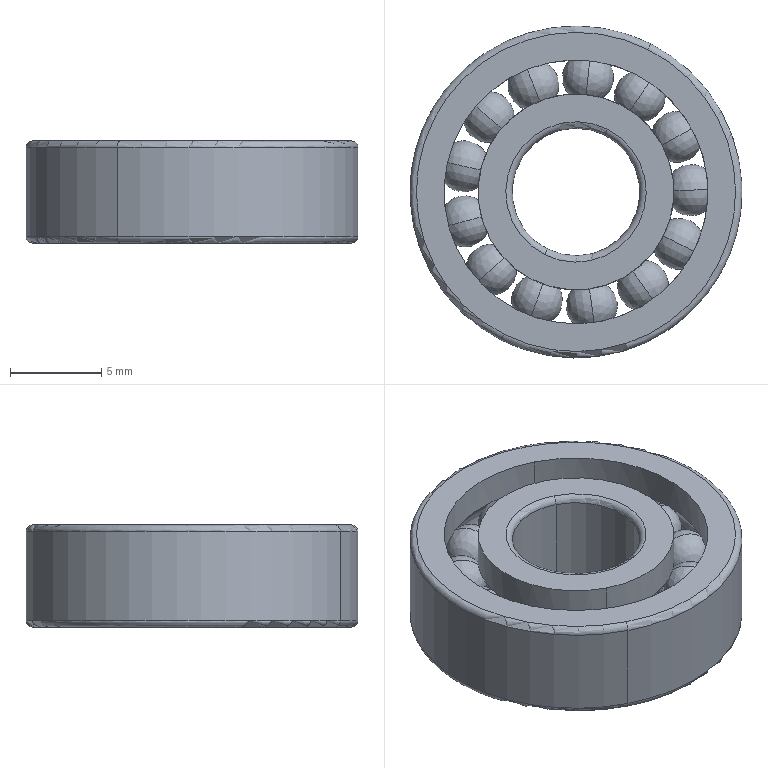Part | SolidWorks | features SplitBody 1 | 1 solid | 92 faces | box 18.2 x 18.2 x 5.6 mm | volume 920.646 mm3 | torus 50 | sphere 26 | cylinder 12 | plane 4 | commonest cylinder face diameters 10.733 x4 14.467 x4 7 x2 18.2 x2